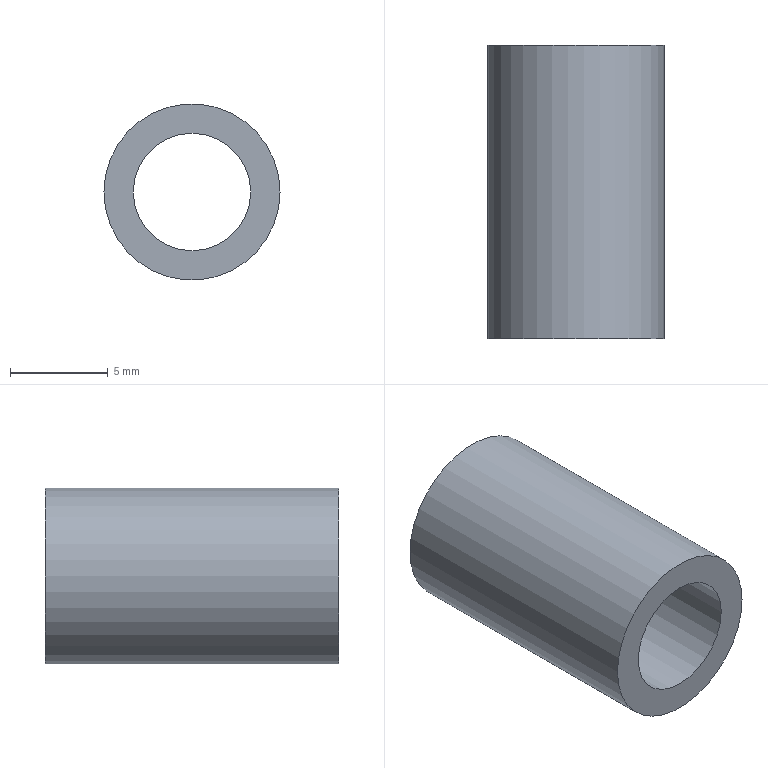Part | STEP file | 1-54.5 | 1 solid | 4 faces | box 9 x 15 x 9 mm | volume 530.144 mm3 | plane 2 | cylinder 2 | commonest cylinder face diameters 6 x1 9 x1
STEP:
#1=CARTESIAN_POINT('',(0.,0.,0.));
#2=DIRECTION('',(0.,0.,1.));
#3=DIRECTION('',(1.,0.,0.));
#4=AXIS2_PLACEMENT_3D('',#1,#2,#3);
#5=CARTESIAN_POINT('',(4.5,0.,0.));
#6=VERTEX_POINT('',#5);
#7=CARTESIAN_POINT('',(0.,0.,0.));
#8=DIRECTION('',(0.,-1.,0.));
#9=DIRECTION('',(1.,0.,0.));
#10=AXIS2_PLACEMENT_3D('',#7,#8,#9);
#11=CIRCLE('',#10,4.5);
#12=CARTESIAN_POINT('',(-1.206,0.,0.));
#13=DIRECTION('',(0.,-1.,0.));
#14=DIRECTION('',(1.,0.,0.));
#15=AXIS2_PLACEMENT_3D('',#12,#13,#14);
#16=PLANE('',#15);
#17=CARTESIAN_POINT('',(1.206,0.));
#18=DIRECTION('',(1.,0.));
#19=AXIS2_PLACEMENT_2D('',#17,#18);
#20=CIRCLE('',#19,4.5);
#21=(GEOMETRIC_REPRESENTATION_CONTEXT(2)PARAMETRIC_REPRESENTATION_CONTEXT()REPRESENTATION_CONTEXT('',''));
#22=DEFINITIONAL_REPRESENTATION('',(#20),#21);
#23=PCURVE('',#16,#22);
#24=CARTESIAN_POINT('',(0.,0.,0.));
#25=DIRECTION('',(0.,1.,0.));
#26=DIRECTION('',(1.,0.,0.));
#27=AXIS2_PLACEMENT_3D('',#24,#25,#26);
#28=CYLINDRICAL_SURFACE('',#27,4.5);
#29=CARTESIAN_POINT('',(6.283,0.));
#30=DIRECTION('',(-1.,0.));
#31=VECTOR('',#30,1.);
#32=LINE('',#29,#31);
#33=(GEOMETRIC_REPRESENTATION_CONTEXT(2)PARAMETRIC_REPRESENTATION_CONTEXT()REPRESENTATION_CONTEXT('',''));
#34=DEFINITIONAL_REPRESENTATION('',(#32),#33);
#35=PCURVE('',#28,#34);
#36=SURFACE_CURVE('',#11,(#23,#35),.PCURVE_S1.);
#37=EDGE_CURVE('',#6,#6,#36,.T.);
#38=ORIENTED_EDGE('',*,*,#37,.T.);
#39=EDGE_LOOP('',(#38));
#40=FACE_BOUND('',#39,.T.);
#41=CARTESIAN_POINT('',(3.,0.,0.));
#42=VERTEX_POINT('',#41);
#43=CARTESIAN_POINT('',(0.,0.,0.));
#44=DIRECTION('',(0.,1.,0.));
#45=DIRECTION('',(1.,0.,0.));
#46=AXIS2_PLACEMENT_3D('',#43,#44,#45);
#47=CIRCLE('',#46,3.);
#48=CARTESIAN_POINT('',(4.206,0.));
#49=CARTESIAN_POINT('',(4.206,-5.196));
#50=CARTESIAN_POINT('',(-0.2942,-2.598));
#51=CARTESIAN_POINT('',(-4.794,0.));
#52=CARTESIAN_POINT('',(-0.2942,2.598));
#53=CARTESIAN_POINT('',(4.206,5.196));
#54=CARTESIAN_POINT('',(4.206,0.));
#55=(BOUNDED_CURVE()B_SPLINE_CURVE(2,(#48,#49,#50,#51,#52,#53,#54),.UNSPECIFIED.,.T.,.F.)B_SPLINE_CURVE_WITH_KNOTS((1,2,2,2,2,1),(-2.094,0.,2.094,4.189,6.283,8.378),.UNSPECIFIED.)CURVE()GEOMETRIC_REPRESENTATION_ITEM()RATIONAL_B_SPLINE_CURVE((1.,0.5,1.,0.5,1.,0.5,1.))REPRESENTATION_ITEM(''));
#56=(GEOMETRIC_REPRESENTATION_CONTEXT(2)PARAMETRIC_REPRESENTATION_CONTEXT()REPRESENTATION_CONTEXT('',''));
#57=DEFINITIONAL_REPRESENTATION('',(#55),#56);
#58=PCURVE('',#16,#57);
#59=CARTESIAN_POINT('',(0.,0.,0.));
#60=DIRECTION('',(0.,1.,0.));
#61=DIRECTION('',(1.,0.,0.));
#62=AXIS2_PLACEMENT_3D('',#59,#60,#61);
#63=CYLINDRICAL_SURFACE('',#62,3.);
#64=CARTESIAN_POINT('',(0.,0.));
#65=DIRECTION('',(1.,0.));
#66=VECTOR('',#65,1.);
#67=LINE('',#64,#66);
#68=(GEOMETRIC_REPRESENTATION_CONTEXT(2)PARAMETRIC_REPRESENTATION_CONTEXT()REPRESENTATION_CONTEXT('',''));
#69=DEFINITIONAL_REPRESENTATION('',(#67),#68);
#70=PCURVE('',#63,#69);
#71=SURFACE_CURVE('',#47,(#58,#70),.PCURVE_S1.);
#72=EDGE_CURVE('',#42,#42,#71,.T.);
#73=ORIENTED_EDGE('',*,*,#72,.T.);
#74=EDGE_LOOP('',(#73));
#75=FACE_BOUND('',#74,.T.);
#76=ADVANCED_FACE('',(#40,#75),#16,.T.);
#77=CARTESIAN_POINT('',(4.5,15.,0.));
#78=VERTEX_POINT('',#77);
#79=CARTESIAN_POINT('',(0.,15.,0.));
#80=DIRECTION('',(0.,-1.,0.));
#81=DIRECTION('',(1.,0.,0.));
#82=AXIS2_PLACEMENT_3D('',#79,#80,#81);
#83=CIRCLE('',#82,4.5);
#84=CARTESIAN_POINT('',(-1.206,15.,0.));
#85=DIRECTION('',(0.,-1.,0.));
#86=DIRECTION('',(1.,0.,0.));
#87=AXIS2_PLACEMENT_3D('',#84,#85,#86);
#88=PLANE('',#87);
#89=CARTESIAN_POINT('',(1.206,0.));
#90=DIRECTION('',(1.,0.));
#91=AXIS2_PLACEMENT_2D('',#89,#90);
#92=CIRCLE('',#91,4.5);
#93=(GEOMETRIC_REPRESENTATION_CONTEXT(2)PARAMETRIC_REPRESENTATION_CONTEXT()REPRESENTATION_CONTEXT('',''));
#94=DEFINITIONAL_REPRESENTATION('',(#92),#93);
#95=PCURVE('',#88,#94);
#96=CARTESIAN_POINT('',(6.283,15.));
#97=DIRECTION('',(-1.,0.));
#98=VECTOR('',#97,1.);
#99=LINE('',#96,#98);
#100=(GEOMETRIC_REPRESENTATION_CONTEXT(2)PARAMETRIC_REPRESENTATION_CONTEXT()REPRESENTATION_CONTEXT('',''));
#101=DEFINITIONAL_REPRESENTATION('',(#99),#100);
#102=PCURVE('',#28,#101);
#103=SURFACE_CURVE('',#83,(#95,#102),.PCURVE_S1.);
#104=EDGE_CURVE('',#78,#78,#103,.T.);
#105=ORIENTED_EDGE('',*,*,#104,.T.);
#106=EDGE_LOOP('',(#105));
#107=FACE_BOUND('',#106,.F.);
#108=CARTESIAN_POINT('',(3.,15.,0.));
#109=VERTEX_POINT('',#108);
#110=CARTESIAN_POINT('',(0.,15.,0.));
#111=DIRECTION('',(0.,1.,0.));
#112=DIRECTION('',(1.,0.,0.));
#113=AXIS2_PLACEMENT_3D('',#110,#111,#112);
#114=CIRCLE('',#113,3.);
#115=CARTESIAN_POINT('',(4.206,0.));
#116=CARTESIAN_POINT('',(4.206,-5.196));
#117=CARTESIAN_POINT('',(-0.2942,-2.598));
#118=CARTESIAN_POINT('',(-4.794,0.));
#119=CARTESIAN_POINT('',(-0.2942,2.598));
#120=CARTESIAN_POINT('',(4.206,5.196));
#121=CARTESIAN_POINT('',(4.206,0.));
#122=(BOUNDED_CURVE()B_SPLINE_CURVE(2,(#115,#116,#117,#118,#119,#120,#121),.UNSPECIFIED.,.T.,.F.)B_SPLINE_CURVE_WITH_KNOTS((1,2,2,2,2,1),(-2.094,0.,2.094,4.189,6.283,8.378),.UNSPECIFIED.)CURVE()GEOMETRIC_REPRESENTATION_ITEM()RATIONAL_B_SPLINE_CURVE((1.,0.5,1.,0.5,1.,0.5,1.))REPRESENTATION_ITEM(''));
#123=(GEOMETRIC_REPRESENTATION_CONTEXT(2)PARAMETRIC_REPRESENTATION_CONTEXT()REPRESENTATION_CONTEXT('',''));
#124=DEFINITIONAL_REPRESENTATION('',(#122),#123);
#125=PCURVE('',#88,#124);
#126=CARTESIAN_POINT('',(0.,15.));
#127=DIRECTION('',(1.,0.));
#128=VECTOR('',#127,1.);
#129=LINE('',#126,#128);
#130=(GEOMETRIC_REPRESENTATION_CONTEXT(2)PARAMETRIC_REPRESENTATION_CONTEXT()REPRESENTATION_CONTEXT('',''));
#131=DEFINITIONAL_REPRESENTATION('',(#129),#130);
#132=PCURVE('',#63,#131);
#133=SURFACE_CURVE('',#114,(#125,#132),.PCURVE_S1.);
#134=EDGE_CURVE('',#109,#109,#133,.T.);
#135=ORIENTED_EDGE('',*,*,#134,.T.);
#136=EDGE_LOOP('',(#135));
#137=FACE_BOUND('',#136,.F.);
#138=ADVANCED_FACE('',(#107,#137),#88,.F.);
#139=CARTESIAN_POINT('',(4.5,0.,0.));
#140=DIRECTION('',(0.,1.,0.));
#141=VECTOR('',#140,1.);
#142=LINE('',#139,#141);
#143=CARTESIAN_POINT('',(6.283,0.));
#144=DIRECTION('',(0.,1.));
#145=VECTOR('',#144,1.);
#146=LINE('',#143,#145);
#147=(GEOMETRIC_REPRESENTATION_CONTEXT(2)PARAMETRIC_REPRESENTATION_CONTEXT()REPRESENTATION_CONTEXT('',''));
#148=DEFINITIONAL_REPRESENTATION('',(#146),#147);
#149=PCURVE('',#28,#148);
#150=CARTESIAN_POINT('',(0.,0.));
#151=DIRECTION('',(0.,1.));
#152=VECTOR('',#151,1.);
#153=LINE('',#150,#152);
#154=(GEOMETRIC_REPRESENTATION_CONTEXT(2)PARAMETRIC_REPRESENTATION_CONTEXT()REPRESENTATION_CONTEXT('',''));
#155=DEFINITIONAL_REPRESENTATION('',(#153),#154);
#156=PCURVE('',#28,#155);
#157=SEAM_CURVE('',#142,(#149,#156),.PCURVE_S1.);
#158=EDGE_CURVE('',#6,#78,#157,.T.);
#159=ORIENTED_EDGE('',*,*,#158,.T.);
#160=ORIENTED_EDGE('',*,*,#104,.T.);
#161=ORIENTED_EDGE('',*,*,#158,.F.);
#162=ORIENTED_EDGE('',*,*,#37,.F.);
#163=EDGE_LOOP('',(#159,#160,#161,#162));
#164=FACE_BOUND('',#163,.T.);
#165=ADVANCED_FACE('',(#164),#28,.T.);
#166=ORIENTED_EDGE('',*,*,#72,.T.);
#167=CARTESIAN_POINT('',(3.,0.,0.));
#168=DIRECTION('',(0.,1.,0.));
#169=VECTOR('',#168,1.);
#170=LINE('',#167,#169);
#171=CARTESIAN_POINT('',(6.283,0.));
#172=DIRECTION('',(0.,1.));
#173=VECTOR('',#172,1.);
#174=LINE('',#171,#173);
#175=(GEOMETRIC_REPRESENTATION_CONTEXT(2)PARAMETRIC_REPRESENTATION_CONTEXT()REPRESENTATION_CONTEXT('',''));
#176=DEFINITIONAL_REPRESENTATION('',(#174),#175);
#177=PCURVE('',#63,#176);
#178=CARTESIAN_POINT('',(0.,0.));
#179=DIRECTION('',(0.,1.));
#180=VECTOR('',#179,1.);
#181=LINE('',#178,#180);
#182=(GEOMETRIC_REPRESENTATION_CONTEXT(2)PARAMETRIC_REPRESENTATION_CONTEXT()REPRESENTATION_CONTEXT('',''));
#183=DEFINITIONAL_REPRESENTATION('',(#181),#182);
#184=PCURVE('',#63,#183);
#185=SEAM_CURVE('',#170,(#177,#184),.PCURVE_S1.);
#186=EDGE_CURVE('',#42,#109,#185,.T.);
#187=ORIENTED_EDGE('',*,*,#186,.T.);
#188=ORIENTED_EDGE('',*,*,#134,.F.);
#189=ORIENTED_EDGE('',*,*,#186,.F.);
#190=EDGE_LOOP('',(#166,#187,#188,#189));
#191=FACE_BOUND('',#190,.F.);
#192=ADVANCED_FACE('',(#191),#63,.F.);
#193=CLOSED_SHELL('',(#76,#138,#165,#192));
#194=MANIFOLD_SOLID_BREP('',#193);
#195=(LENGTH_UNIT()NAMED_UNIT(*)SI_UNIT(.MILLI.,.METRE.));
#196=UNCERTAINTY_MEASURE_WITH_UNIT(LENGTH_MEASURE(0.0000001),#195,'','');
#197=(NAMED_UNIT(*)PLANE_ANGLE_UNIT()SI_UNIT($,.RADIAN.));
#198=(NAMED_UNIT(*)SI_UNIT($,.STERADIAN.)SOLID_ANGLE_UNIT());
#199=(GEOMETRIC_REPRESENTATION_CONTEXT(3)GLOBAL_UNCERTAINTY_ASSIGNED_CONTEXT((#196))GLOBAL_UNIT_ASSIGNED_CONTEXT((#195,#197,#198))REPRESENTATION_CONTEXT('',''));
#200=ADVANCED_BREP_SHAPE_REPRESENTATION('',(#4,#194),#199);